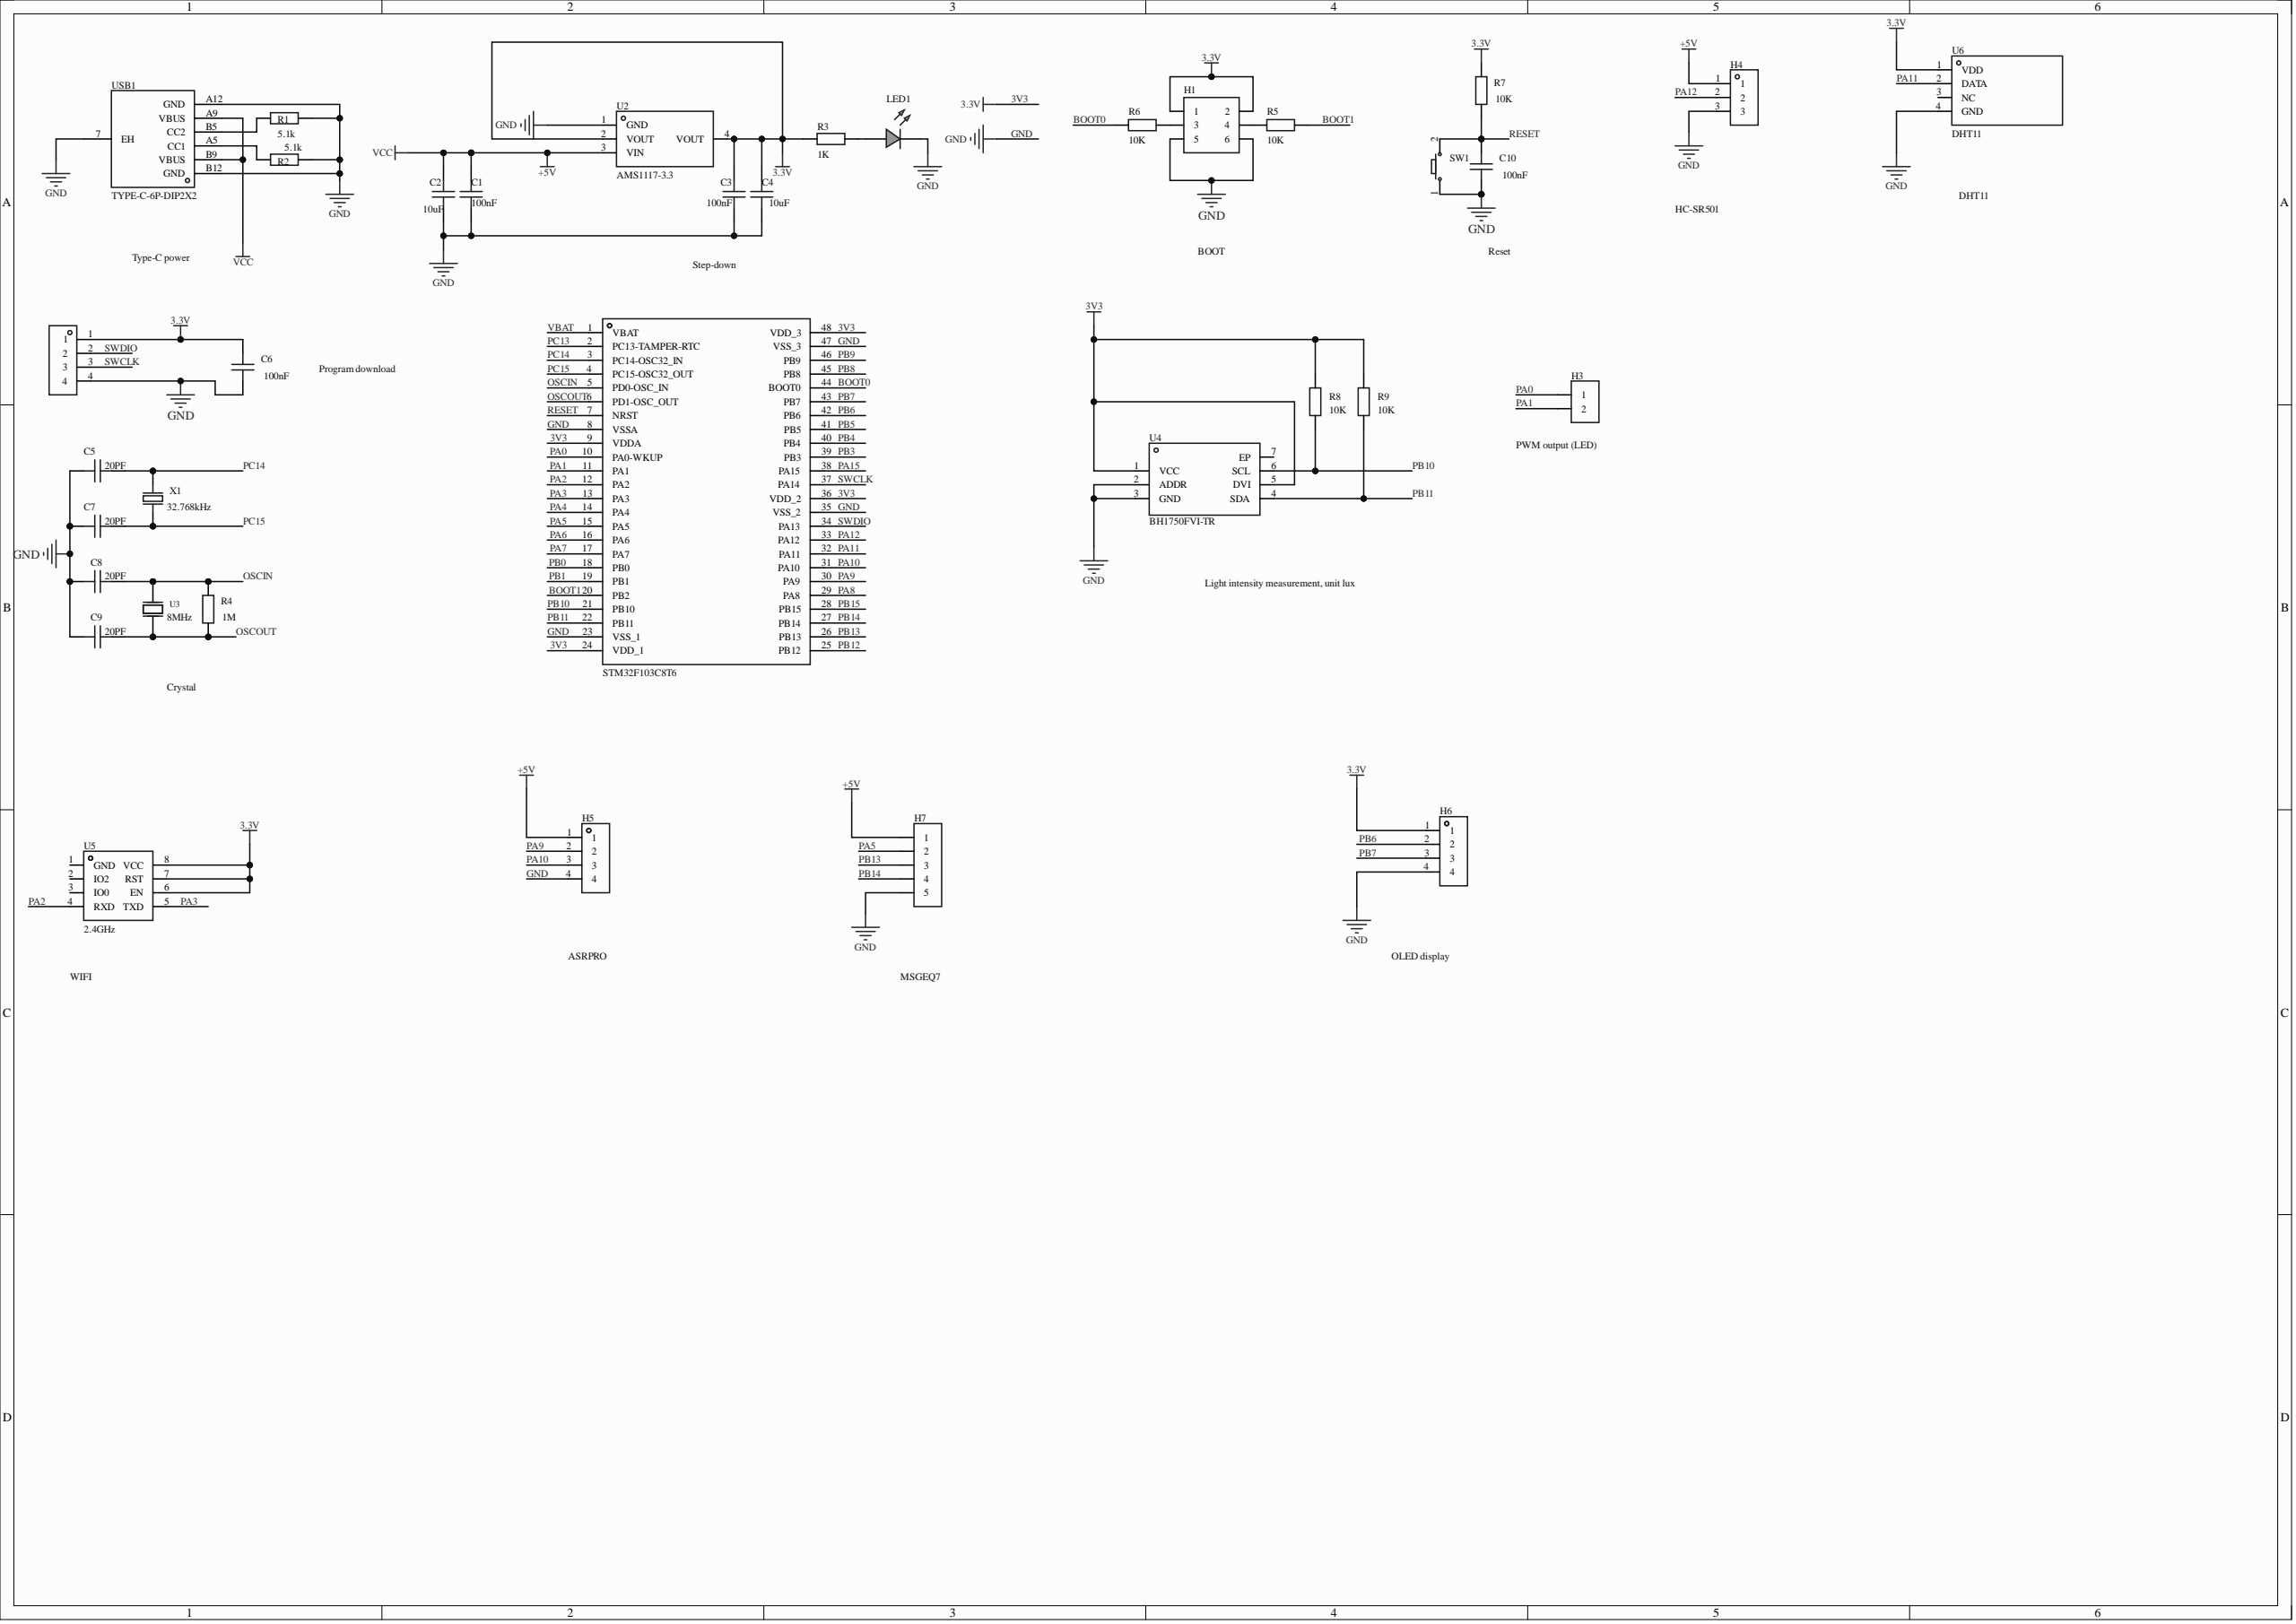Circuit board | Altium Designer | 36 parts | 32 nets
Bill of materials:
Comment,Description,Designator,Footprint,LibRef,Quantity
"100nF","","C1, C3, C6, C10","C0805","CAP_0805","4"
"10uF","","C2, C4","C0805","CAP_0805","2"
"20PF","","C5, C7, C8, C9","C0805","CAP_0805","4"
"","","H1","HDR-TH_6P-P2.54-V-R2-C3-S2.54_A2541WV-2X3P","HDR-M_2.54_2x3","1"
"","","H2","HDR-TH_4P-P2.54-V-M","HDR-M_2.54_1x4P","1"
"","","H3","HDR-TH_2P-P2.54-V-F","HDR-F_2.54_1x2P","1"
"","","H4","HDR-TH_3P-P2.54-V-F","HDR-F_2.54_1x3P","1"
"","","H5, H6","HDR-TH_4P-P2.54-V-F","HDR-F_2.54_1x4P","2"
"","","H7","HDR-TH_5P-P2.54-V-F","HDR-F_2.54_1x5P","1"
"","","LED1","LED_0805","LED_0805-G","1"
"5.1k","","R1, R2","R0805","Res_0805","2"
"1K","","R3","R0805","Res_0805","1"
"1M","","R4","R0805","Res_0805","1"
"10K","","R5, R6, R7, R8, R9","R0805","Res_0805","5"
"","","SW1","Key_SMD_3.6x6.1x2.5","Key_SMD_3.6x6.1x2.5","1"
"STM32F103C8T6","CPU core: ARM Cortex-M3; max CPU frequency: 72MHz; program storage capacity: 64KB; program memory type: FLASH; total RAM: 20KB; GPIO port count: 37;","U1","LQFP-48_L7.0-W7.0-P0.50-LS9.0-BL","STM32F103C8T6","1"
"AMS1117-3.3","Output type: fixed; working voltage: 16V; output voltage: 3.3V; output current: 1A; power supply ripple rejection (PSRR): 72dB@(120Hz); output polarity: positive;","U2","SOT-223-3_L6.5-W3.4-P2.30-LS7.0-BR","AMS1117-3.3_C6186","1"
"8MHz","Frequency: 10MHz; frequency tolerance: ±30ppm; load capacitance: 18pF;","U3","CRYSTAL-TH_L10.8-W4.5-P4.88","ATS100B-E","1"
"BH1750FVI-TR","Detection colour: -; interface type: I2C;","U4","WSOF-6_L2.6-W1.6-P0.50-TL-EP","BH1750FVI-TR","1"
"2.4GHz","Core processor: ESP8266 chip; frequency: 2.4GHz; antenna type: onboard PCB antenna; transmit power: 16dBm; receive sensitivity: -90dBm;","U5","WIFIM-TH_8P-L24.7-W14.4-P2.54","ESP-01S","1"
"DHT11","Temperature range: -20℃~+60℃; humidity range: 5%RH~95%RH; humidity accuracy: ±5%RH;","U6","SENSOR-TH_DHT11","DHT11","1"
"TYPE-C-6P-DIP2X2","","USB1","TYPE-C-SMD_TYPE-C-6P","TYPE-C-6P-DIP2X2","1"
"32.768kHz","Frequency: 32.768kHz; frequency tolerance: ±20ppm; load capacitance: 12.5pF;","X1","FC-135R_L3.2-W1.5","Q13FC1350000400","1"
Netlist (Protel format):
[
C1
C0805
100nF



]
[
C2
C0805
10uF



]
[
C3
C0805
100nF



]
[
C4
C0805
10uF



]
[
C5
C0805
20PF



]
[
C6
C0805
100nF



]
[
C7
C0805
20PF



]
[
C8
C0805
20PF



]
[
C9
C0805
20PF



]
[
C10
C0805
100nF



]
[
H1
HDR-TH_6P-P2.54-V-R2-C3-S2.54_A2541WV-2X3P




]
[
H2
HDR-TH_4P-P2.54-V-M




]
[
H3
HDR-TH_2P-P2.54-V-F




]
[
H4
HDR-TH_3P-P2.54-V-F




]
[
H5
HDR-TH_4P-P2.54-V-F




]
[
H6
HDR-TH_4P-P2.54-V-F




]
[
H7
HDR-TH_5P-P2.54-V-F




]
[
LED1
LED_0805




]
[
R1
R0805
5.1k



]
[
R2
R0805
5.1k



]
[
R3
R0805
1K



]
[
R4
R0805
1M



]
[
R5
R0805
10K



]
[
R6
R0805
10K



]
[
R7
R0805
10K



]
[
R8
R0805
10K



]
[
R9
R0805
10K



]
[
SW1
Key_SMD_3.6x6.1x2.5




]
[
U1
LQFP-48_L7.0-W7.0-P0.50-LS9.0-BL
STM32F103C8T6



]
[
U2
SOT-223-3_L6.5-W3.4-P2.30-LS7.0-BR
AMS1117-3.3



]
[
U3
CRYSTAL-TH_L10.8-W4.5-P4.88
8MHz



]
[
U4
WSOF-6_L2.6-W1.6-P0.50-TL-EP
BH1750FVI-TR



]
[
U5
WIFIM-TH_8P-L24.7-W14.4-P2.54
2.4GHz



]
[
U6
SENSOR-TH_DHT11
DHT11



]
[
USB1
TYPE-C-SMD_TYPE-C-6P
TYPE-C-6P-DIP2X2



]
[
X1
FC-135R_L3.2-W1.5
32.768kHz



]
(
SWDIO
H2-2
U1-34
)
(
SWCLK
H2-3
U1-37
)
(
RESET
C10-2
R7-1
SW1-2
U1-7
)
(
PC15
C7-2
U1-4
X1-1
)
(
PC14
C5-1
U1-3
X1-2
)
(
PB14
H7-4
U1-27
)
(
PB13
H7-3
U1-26
)
(
PB11
R9-1
U1-22
U4-4
)
(
PB10
R8-1
U1-21
U4-6
)
(
PB7
H6-3
U1-43
)
(
PB6
H6-2
U1-42
)
(
PA12
H4-2
U1-33
)
(
PA11
U1-32
U6-2
)
(
PA10
H5-3
U1-31
)
(
PA9
H5-2
U1-30
)
(
PA5
H7-2
U1-15
)
(
PA3
U1-13
U5-5
)
(
PA2
U1-12
U5-4
)
(
PA1
H3-2
U1-11
)
(
PA0
H3-1
U1-10
)
(
OSCOUT
C9-1
R4-1
U1-6
U3-1
)
(
OSCIN
C8-1
R4-2
U1-5
U3-2
)
(
NetR2_1
R2-1
USB1-A5
)
(
NetR1_1
R1-1
USB1-B5
)
(
NetLED1_2
LED1-2
R3-2
)
(
NetH1_4
H1-4
R5-1
)
(
NetH1_3
H1-3
R6-2
)
(
GND
C1-1
C2-1
C3-1
C4-1
C5-2
C6-1
C7-1
C8-2
C9-2
C10-1
H1-5
H1-6
H2-4
H4-3
H5-4
H6-4
H7-5
LED1-1
R1-2
R2-2
SW1-1
U1-8
U1-23
U1-35
U1-47
U2-1
U4-2
U4-3
U6-4
USB1-7
USB1-A12
USB1-B12
)
(
BOOT1
R5-2
U1-20
)
(
BOOT0
R6-1
U1-44
)
(
+5V
C1-2
C2-2
H4-1
H5-1
H7-1
U2-3
USB1-A9
USB1-B9
)
(
3V3
C3-2
C4-2
C6-2
H1-1
H1-2
H2-1
H6-1
R3-1
R7-2
R8-2
R9-2
U1-9
U1-24
U1-36
U1-48
U2-2
U2-4
U4-1
U4-5
U5-6
U5-7
U5-8
U6-1
)